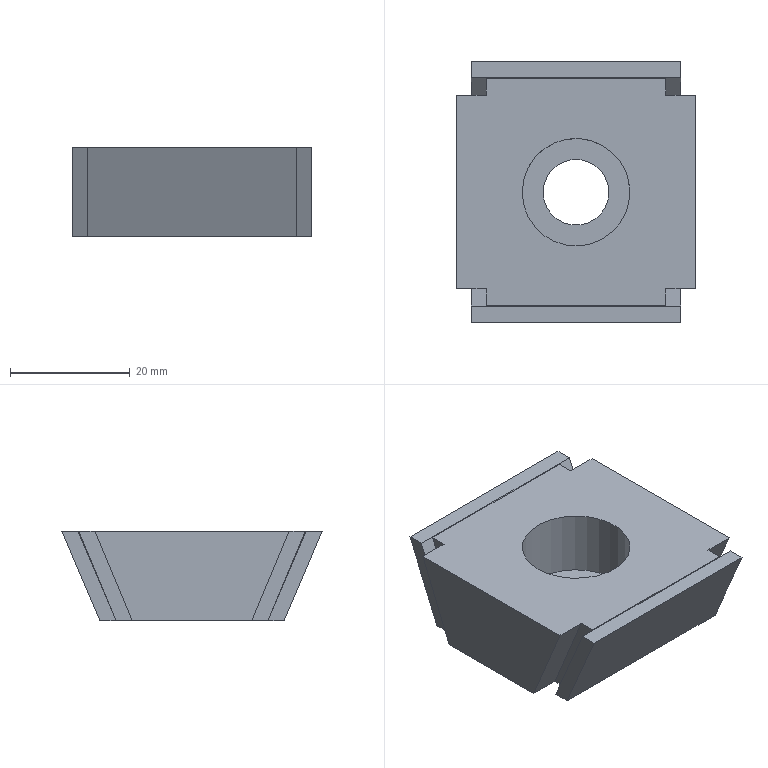Part | NX | features DATUM_CSYS 5, SKETCH 4, EXTRUDE 3, CBORE_HOLE 1, HOLE PACKAGE 1 | 3 solids | 29 faces | box 40 x 43.514 x 15 mm | volume 17811 mm3 | plane 27 | cylinder 2 | commonest cylinder face diameters 11 x1 18 x1
STEP:
#1=CARTESIAN_POINT('',(-40.,0.,0.));
#2=VERTEX_POINT('',#1);
#3=CARTESIAN_POINT('',(-35.,0.,0.));
#4=VERTEX_POINT('',#3);
#5=CARTESIAN_POINT('',(-40.,0.,0.));
#6=DIRECTION('',(1.,0.,0.));
#7=VECTOR('',#6,1000.);
#8=LINE('',#5,#7);
#9=EDGE_CURVE('',#2,#4,#8,.T.);
#10=ORIENTED_EDGE('',*,*,#9,.T.);
#11=CARTESIAN_POINT('',(-35.,-6.213,15.));
#12=VERTEX_POINT('',#11);
#13=CARTESIAN_POINT('',(-35.,0.,0.));
#14=DIRECTION('',(0.,-0.3827,0.9239));
#15=VECTOR('',#14,1000.);
#16=LINE('',#13,#15);
#17=EDGE_CURVE('',#4,#12,#16,.T.);
#18=ORIENTED_EDGE('',*,*,#17,.T.);
#19=CARTESIAN_POINT('',(-40.,-6.213,15.));
#20=VERTEX_POINT('',#19);
#21=CARTESIAN_POINT('',(-40.,-6.213,15.));
#22=DIRECTION('',(1.,0.,0.));
#23=VECTOR('',#22,1000.);
#24=LINE('',#21,#23);
#25=EDGE_CURVE('',#20,#12,#24,.T.);
#26=ORIENTED_EDGE('',*,*,#25,.F.);
#27=CARTESIAN_POINT('',(-40.,-6.213,15.));
#28=DIRECTION('',(0.,0.3827,-0.9239));
#29=VECTOR('',#28,1000.);
#30=LINE('',#27,#29);
#31=EDGE_CURVE('',#20,#2,#30,.T.);
#32=ORIENTED_EDGE('',*,*,#31,.T.);
#33=EDGE_LOOP('',(#10,#18,#26,#32));
#34=FACE_BOUND('',#33,.T.);
#35=CARTESIAN_POINT('',(-40.,-6.213,15.));
#36=DIRECTION('',(0.,-0.9239,-0.3827));
#37=DIRECTION('',(0.,0.3827,-0.9239));
#38=AXIS2_PLACEMENT_3D('',#35,#36,#37);
#39=PLANE('',#38);
#40=ADVANCED_FACE('',(#34),#39,.T.);
#41=CARTESIAN_POINT('',(-40.,26.213,15.));
#42=VERTEX_POINT('',#41);
#43=CARTESIAN_POINT('',(-35.,26.213,15.));
#44=VERTEX_POINT('',#43);
#45=CARTESIAN_POINT('',(-40.,26.213,15.));
#46=DIRECTION('',(1.,0.,0.));
#47=VECTOR('',#46,1000.);
#48=LINE('',#45,#47);
#49=EDGE_CURVE('',#42,#44,#48,.T.);
#50=ORIENTED_EDGE('',*,*,#49,.T.);
#51=CARTESIAN_POINT('',(-35.,20.,0.));
#52=VERTEX_POINT('',#51);
#53=CARTESIAN_POINT('',(-35.,26.213,15.));
#54=DIRECTION('',(0.,-0.3827,-0.9239));
#55=VECTOR('',#54,1000.);
#56=LINE('',#53,#55);
#57=EDGE_CURVE('',#44,#52,#56,.T.);
#58=ORIENTED_EDGE('',*,*,#57,.T.);
#59=CARTESIAN_POINT('',(-40.,20.,0.));
#60=VERTEX_POINT('',#59);
#61=CARTESIAN_POINT('',(-40.,20.,0.));
#62=DIRECTION('',(1.,0.,0.));
#63=VECTOR('',#62,1000.);
#64=LINE('',#61,#63);
#65=EDGE_CURVE('',#60,#52,#64,.T.);
#66=ORIENTED_EDGE('',*,*,#65,.F.);
#67=CARTESIAN_POINT('',(-40.,20.,0.));
#68=DIRECTION('',(0.,0.3827,0.9239));
#69=VECTOR('',#68,1000.);
#70=LINE('',#67,#69);
#71=EDGE_CURVE('',#60,#42,#70,.T.);
#72=ORIENTED_EDGE('',*,*,#71,.T.);
#73=EDGE_LOOP('',(#50,#58,#66,#72));
#74=FACE_BOUND('',#73,.T.);
#75=CARTESIAN_POINT('',(-40.,20.,0.));
#76=DIRECTION('',(0.,0.9239,-0.3827));
#77=DIRECTION('',(0.,0.3827,0.9239));
#78=AXIS2_PLACEMENT_3D('',#75,#76,#77);
#79=PLANE('',#78);
#80=ADVANCED_FACE('',(#74),#79,.T.);
#81=CARTESIAN_POINT('',(-5.,0.,0.));
#82=VERTEX_POINT('',#81);
#83=CARTESIAN_POINT('',(-5.,-6.213,15.));
#84=VERTEX_POINT('',#83);
#85=CARTESIAN_POINT('',(-5.,0.,0.));
#86=DIRECTION('',(0.,-0.3827,0.9239));
#87=VECTOR('',#86,1000.);
#88=LINE('',#85,#87);
#89=EDGE_CURVE('',#82,#84,#88,.T.);
#90=ORIENTED_EDGE('',*,*,#89,.F.);
#91=CARTESIAN_POINT('',(0.,0.,0.));
#92=VERTEX_POINT('',#91);
#93=CARTESIAN_POINT('',(-40.,0.,0.));
#94=DIRECTION('',(1.,0.,0.));
#95=VECTOR('',#94,1000.);
#96=LINE('',#93,#95);
#97=EDGE_CURVE('',#82,#92,#96,.T.);
#98=ORIENTED_EDGE('',*,*,#97,.T.);
#99=CARTESIAN_POINT('',(0.,-6.213,15.));
#100=VERTEX_POINT('',#99);
#101=CARTESIAN_POINT('',(0.,-6.213,15.));
#102=DIRECTION('',(0.,0.3827,-0.9239));
#103=VECTOR('',#102,1000.);
#104=LINE('',#101,#103);
#105=EDGE_CURVE('',#100,#92,#104,.T.);
#106=ORIENTED_EDGE('',*,*,#105,.F.);
#107=CARTESIAN_POINT('',(-40.,-6.213,15.));
#108=DIRECTION('',(1.,0.,0.));
#109=VECTOR('',#108,1000.);
#110=LINE('',#107,#109);
#111=EDGE_CURVE('',#84,#100,#110,.T.);
#112=ORIENTED_EDGE('',*,*,#111,.F.);
#113=EDGE_LOOP('',(#90,#98,#106,#112));
#114=FACE_BOUND('',#113,.T.);
#115=CARTESIAN_POINT('',(-40.,-6.213,15.));
#116=DIRECTION('',(0.,-0.9239,-0.3827));
#117=DIRECTION('',(0.,0.3827,-0.9239));
#118=AXIS2_PLACEMENT_3D('',#115,#116,#117);
#119=PLANE('',#118);
#120=ADVANCED_FACE('',(#114),#119,.T.);
#121=CARTESIAN_POINT('',(-25.5,9.963,0.));
#122=VERTEX_POINT('',#121);
#123=CARTESIAN_POINT('',(-20.,9.963,0.));
#124=DIRECTION('',(0.,0.,-1.));
#125=DIRECTION('',(-1.,0.,0.));
#126=AXIS2_PLACEMENT_3D('',#123,#124,#125);
#127=CIRCLE('',#126,5.5);
#128=EDGE_CURVE('',#122,#122,#127,.T.);
#129=ORIENTED_EDGE('',*,*,#128,.F.);
#130=EDGE_LOOP('',(#129));
#131=FACE_BOUND('',#130,.T.);
#132=CARTESIAN_POINT('',(0.,20.,0.));
#133=VERTEX_POINT('',#132);
#134=CARTESIAN_POINT('',(0.,0.,0.));
#135=DIRECTION('',(0.,1.,0.));
#136=VECTOR('',#135,1000.);
#137=LINE('',#134,#136);
#138=EDGE_CURVE('',#92,#133,#137,.T.);
#139=ORIENTED_EDGE('',*,*,#138,.F.);
#140=ORIENTED_EDGE('',*,*,#97,.F.);
#141=CARTESIAN_POINT('',(-5.,-2.7,0.));
#142=VERTEX_POINT('',#141);
#143=CARTESIAN_POINT('',(-5.,-2.7,0.));
#144=DIRECTION('',(0.,1.,0.));
#145=VECTOR('',#144,1000.);
#146=LINE('',#143,#145);
#147=EDGE_CURVE('',#142,#82,#146,.T.);
#148=ORIENTED_EDGE('',*,*,#147,.F.);
#149=CARTESIAN_POINT('',(-35.,-2.7,0.));
#150=VERTEX_POINT('',#149);
#151=CARTESIAN_POINT('',(-35.,-2.7,0.));
#152=DIRECTION('',(1.,0.,0.));
#153=VECTOR('',#152,1000.);
#154=LINE('',#151,#153);
#155=EDGE_CURVE('',#150,#142,#154,.T.);
#156=ORIENTED_EDGE('',*,*,#155,.F.);
#157=CARTESIAN_POINT('',(-35.,-2.7,0.));
#158=DIRECTION('',(0.,1.,0.));
#159=VECTOR('',#158,1000.);
#160=LINE('',#157,#159);
#161=EDGE_CURVE('',#150,#4,#160,.T.);
#162=ORIENTED_EDGE('',*,*,#161,.T.);
#163=ORIENTED_EDGE('',*,*,#9,.F.);
#164=CARTESIAN_POINT('',(-40.,0.,0.));
#165=DIRECTION('',(0.,1.,0.));
#166=VECTOR('',#165,1000.);
#167=LINE('',#164,#166);
#168=EDGE_CURVE('',#2,#60,#167,.T.);
#169=ORIENTED_EDGE('',*,*,#168,.T.);
#170=ORIENTED_EDGE('',*,*,#65,.T.);
#171=CARTESIAN_POINT('',(-35.,22.7,0.));
#172=VERTEX_POINT('',#171);
#173=CARTESIAN_POINT('',(-35.,20.,0.));
#174=DIRECTION('',(0.,1.,0.));
#175=VECTOR('',#174,1000.);
#176=LINE('',#173,#175);
#177=EDGE_CURVE('',#52,#172,#176,.T.);
#178=ORIENTED_EDGE('',*,*,#177,.T.);
#179=CARTESIAN_POINT('',(-5.,22.7,0.));
#180=VERTEX_POINT('',#179);
#181=CARTESIAN_POINT('',(-35.,22.7,0.));
#182=DIRECTION('',(1.,0.,0.));
#183=VECTOR('',#182,1000.);
#184=LINE('',#181,#183);
#185=EDGE_CURVE('',#172,#180,#184,.T.);
#186=ORIENTED_EDGE('',*,*,#185,.T.);
#187=CARTESIAN_POINT('',(-5.,20.,0.));
#188=VERTEX_POINT('',#187);
#189=CARTESIAN_POINT('',(-5.,20.,0.));
#190=DIRECTION('',(0.,1.,0.));
#191=VECTOR('',#190,1000.);
#192=LINE('',#189,#191);
#193=EDGE_CURVE('',#188,#180,#192,.T.);
#194=ORIENTED_EDGE('',*,*,#193,.F.);
#195=CARTESIAN_POINT('',(-40.,20.,0.));
#196=DIRECTION('',(1.,0.,0.));
#197=VECTOR('',#196,1000.);
#198=LINE('',#195,#197);
#199=EDGE_CURVE('',#188,#133,#198,.T.);
#200=ORIENTED_EDGE('',*,*,#199,.T.);
#201=EDGE_LOOP('',(#139,#140,#148,#156,#162,#163,#169,#170,#178,#186,#194,#200));
#202=FACE_BOUND('',#201,.T.);
#203=CARTESIAN_POINT('',(-40.,0.,0.));
#204=DIRECTION('',(0.,0.,-1.));
#205=DIRECTION('',(-1.,0.,0.));
#206=AXIS2_PLACEMENT_3D('',#203,#204,#205);
#207=PLANE('',#206);
#208=ADVANCED_FACE('',(#131,#202),#207,.T.);
#209=CARTESIAN_POINT('',(-5.,26.213,15.));
#210=VERTEX_POINT('',#209);
#211=CARTESIAN_POINT('',(-5.,26.213,15.));
#212=DIRECTION('',(0.,-0.3827,-0.9239));
#213=VECTOR('',#212,1000.);
#214=LINE('',#211,#213);
#215=EDGE_CURVE('',#210,#188,#214,.T.);
#216=ORIENTED_EDGE('',*,*,#215,.F.);
#217=CARTESIAN_POINT('',(0.,26.213,15.));
#218=VERTEX_POINT('',#217);
#219=CARTESIAN_POINT('',(-40.,26.213,15.));
#220=DIRECTION('',(1.,0.,0.));
#221=VECTOR('',#220,1000.);
#222=LINE('',#219,#221);
#223=EDGE_CURVE('',#210,#218,#222,.T.);
#224=ORIENTED_EDGE('',*,*,#223,.T.);
#225=CARTESIAN_POINT('',(0.,20.,0.));
#226=DIRECTION('',(0.,0.3827,0.9239));
#227=VECTOR('',#226,1000.);
#228=LINE('',#225,#227);
#229=EDGE_CURVE('',#133,#218,#228,.T.);
#230=ORIENTED_EDGE('',*,*,#229,.F.);
#231=ORIENTED_EDGE('',*,*,#199,.F.);
#232=EDGE_LOOP('',(#216,#224,#230,#231));
#233=FACE_BOUND('',#232,.T.);
#234=CARTESIAN_POINT('',(-40.,20.,0.));
#235=DIRECTION('',(0.,0.9239,-0.3827));
#236=DIRECTION('',(0.,0.3827,0.9239));
#237=AXIS2_PLACEMENT_3D('',#234,#235,#236);
#238=PLANE('',#237);
#239=ADVANCED_FACE('',(#233),#238,.T.);
#240=CARTESIAN_POINT('',(-29.,9.963,15.));
#241=VERTEX_POINT('',#240);
#242=CARTESIAN_POINT('',(-20.,9.963,15.));
#243=DIRECTION('',(0.,0.,-1.));
#244=DIRECTION('',(-1.,0.,0.));
#245=AXIS2_PLACEMENT_3D('',#242,#243,#244);
#246=CIRCLE('',#245,9.);
#247=EDGE_CURVE('',#241,#241,#246,.T.);
#248=ORIENTED_EDGE('',*,*,#247,.T.);
#249=EDGE_LOOP('',(#248));
#250=FACE_BOUND('',#249,.T.);
#251=CARTESIAN_POINT('',(0.,26.213,15.));
#252=DIRECTION('',(0.,-1.,0.));
#253=VECTOR('',#252,1000.);
#254=LINE('',#251,#253);
#255=EDGE_CURVE('',#218,#100,#254,.T.);
#256=ORIENTED_EDGE('',*,*,#255,.F.);
#257=ORIENTED_EDGE('',*,*,#223,.F.);
#258=CARTESIAN_POINT('',(-5.,28.913,15.));
#259=VERTEX_POINT('',#258);
#260=CARTESIAN_POINT('',(-5.,28.913,15.));
#261=DIRECTION('',(0.,-1.,0.));
#262=VECTOR('',#261,1000.);
#263=LINE('',#260,#262);
#264=EDGE_CURVE('',#259,#210,#263,.T.);
#265=ORIENTED_EDGE('',*,*,#264,.F.);
#266=CARTESIAN_POINT('',(-35.,28.913,15.));
#267=VERTEX_POINT('',#266);
#268=CARTESIAN_POINT('',(-35.,28.913,15.));
#269=DIRECTION('',(1.,0.,0.));
#270=VECTOR('',#269,1000.);
#271=LINE('',#268,#270);
#272=EDGE_CURVE('',#267,#259,#271,.T.);
#273=ORIENTED_EDGE('',*,*,#272,.F.);
#274=CARTESIAN_POINT('',(-35.,28.913,15.));
#275=DIRECTION('',(0.,-1.,0.));
#276=VECTOR('',#275,1000.);
#277=LINE('',#274,#276);
#278=EDGE_CURVE('',#267,#44,#277,.T.);
#279=ORIENTED_EDGE('',*,*,#278,.T.);
#280=ORIENTED_EDGE('',*,*,#49,.F.);
#281=CARTESIAN_POINT('',(-40.,26.213,15.));
#282=DIRECTION('',(0.,-1.,0.));
#283=VECTOR('',#282,1000.);
#284=LINE('',#281,#283);
#285=EDGE_CURVE('',#42,#20,#284,.T.);
#286=ORIENTED_EDGE('',*,*,#285,.T.);
#287=ORIENTED_EDGE('',*,*,#25,.T.);
#288=CARTESIAN_POINT('',(-35.,-8.913,15.));
#289=VERTEX_POINT('',#288);
#290=CARTESIAN_POINT('',(-35.,-6.213,15.));
#291=DIRECTION('',(0.,-1.,0.));
#292=VECTOR('',#291,1000.);
#293=LINE('',#290,#292);
#294=EDGE_CURVE('',#12,#289,#293,.T.);
#295=ORIENTED_EDGE('',*,*,#294,.T.);
#296=CARTESIAN_POINT('',(-5.,-8.913,15.));
#297=VERTEX_POINT('',#296);
#298=CARTESIAN_POINT('',(-35.,-8.913,15.));
#299=DIRECTION('',(1.,0.,0.));
#300=VECTOR('',#299,1000.);
#301=LINE('',#298,#300);
#302=EDGE_CURVE('',#289,#297,#301,.T.);
#303=ORIENTED_EDGE('',*,*,#302,.T.);
#304=CARTESIAN_POINT('',(-5.,-6.213,15.));
#305=DIRECTION('',(0.,-1.,0.));
#306=VECTOR('',#305,1000.);
#307=LINE('',#304,#306);
#308=EDGE_CURVE('',#84,#297,#307,.T.);
#309=ORIENTED_EDGE('',*,*,#308,.F.);
#310=ORIENTED_EDGE('',*,*,#111,.T.);
#311=EDGE_LOOP('',(#256,#257,#265,#273,#279,#280,#286,#287,#295,#303,#309,#310));
#312=FACE_BOUND('',#311,.T.);
#313=CARTESIAN_POINT('',(-40.,26.213,15.));
#314=DIRECTION('',(0.,0.,1.));
#315=DIRECTION('',(1.,0.,0.));
#316=AXIS2_PLACEMENT_3D('',#313,#314,#315);
#317=PLANE('',#316);
#318=ADVANCED_FACE('',(#250,#312),#317,.T.);
#319=ORIENTED_EDGE('',*,*,#31,.F.);
#320=ORIENTED_EDGE('',*,*,#285,.F.);
#321=ORIENTED_EDGE('',*,*,#71,.F.);
#322=ORIENTED_EDGE('',*,*,#168,.F.);
#323=EDGE_LOOP('',(#319,#320,#321,#322));
#324=FACE_BOUND('',#323,.T.);
#325=CARTESIAN_POINT('',(-40.,0.,0.));
#326=DIRECTION('',(1.,0.,0.));
#327=DIRECTION('',(0.,0.,-1.));
#328=AXIS2_PLACEMENT_3D('',#325,#326,#327);
#329=PLANE('',#328);
#330=ADVANCED_FACE('',(#324),#329,.F.);
#331=ORIENTED_EDGE('',*,*,#105,.T.);
#332=ORIENTED_EDGE('',*,*,#138,.T.);
#333=ORIENTED_EDGE('',*,*,#229,.T.);
#334=ORIENTED_EDGE('',*,*,#255,.T.);
#335=EDGE_LOOP('',(#331,#332,#333,#334));
#336=FACE_BOUND('',#335,.T.);
#337=CARTESIAN_POINT('',(0.,0.,0.));
#338=DIRECTION('',(1.,0.,0.));
#339=DIRECTION('',(0.,0.,-1.));
#340=AXIS2_PLACEMENT_3D('',#337,#338,#339);
#341=PLANE('',#340);
#342=ADVANCED_FACE('',(#336),#341,.T.);
#343=CARTESIAN_POINT('',(-5.,22.7,0.));
#344=DIRECTION('',(0.,0.3827,0.9239));
#345=VECTOR('',#344,1000.);
#346=LINE('',#343,#345);
#347=EDGE_CURVE('',#180,#259,#346,.T.);
#348=ORIENTED_EDGE('',*,*,#347,.F.);
#349=ORIENTED_EDGE('',*,*,#185,.F.);
#350=CARTESIAN_POINT('',(-35.,22.7,0.));
#351=DIRECTION('',(0.,0.3827,0.9239));
#352=VECTOR('',#351,1000.);
#353=LINE('',#350,#352);
#354=EDGE_CURVE('',#172,#267,#353,.T.);
#355=ORIENTED_EDGE('',*,*,#354,.T.);
#356=ORIENTED_EDGE('',*,*,#272,.T.);
#357=EDGE_LOOP('',(#348,#349,#355,#356));
#358=FACE_BOUND('',#357,.T.);
#359=CARTESIAN_POINT('',(-35.,22.7,0.));
#360=DIRECTION('',(0.,0.9239,-0.3827));
#361=DIRECTION('',(0.,0.3827,0.9239));
#362=AXIS2_PLACEMENT_3D('',#359,#360,#361);
#363=PLANE('',#362);
#364=ADVANCED_FACE('',(#358),#363,.T.);
#365=ORIENTED_EDGE('',*,*,#177,.F.);
#366=ORIENTED_EDGE('',*,*,#57,.F.);
#367=ORIENTED_EDGE('',*,*,#278,.F.);
#368=ORIENTED_EDGE('',*,*,#354,.F.);
#369=EDGE_LOOP('',(#365,#366,#367,#368));
#370=FACE_BOUND('',#369,.T.);
#371=CARTESIAN_POINT('',(-35.,0.,0.));
#372=DIRECTION('',(1.,0.,0.));
#373=DIRECTION('',(0.,0.,-1.));
#374=AXIS2_PLACEMENT_3D('',#371,#372,#373);
#375=PLANE('',#374);
#376=ADVANCED_FACE('',(#370),#375,.F.);
#377=ORIENTED_EDGE('',*,*,#193,.T.);
#378=ORIENTED_EDGE('',*,*,#347,.T.);
#379=ORIENTED_EDGE('',*,*,#264,.T.);
#380=ORIENTED_EDGE('',*,*,#215,.T.);
#381=EDGE_LOOP('',(#377,#378,#379,#380));
#382=FACE_BOUND('',#381,.T.);
#383=CARTESIAN_POINT('',(-5.,0.,0.));
#384=DIRECTION('',(1.,0.,0.));
#385=DIRECTION('',(0.,0.,-1.));
#386=AXIS2_PLACEMENT_3D('',#383,#384,#385);
#387=PLANE('',#386);
#388=ADVANCED_FACE('',(#382),#387,.T.);
#389=CARTESIAN_POINT('',(-5.,-8.913,15.));
#390=DIRECTION('',(0.,0.3827,-0.9239));
#391=VECTOR('',#390,1000.);
#392=LINE('',#389,#391);
#393=EDGE_CURVE('',#297,#142,#392,.T.);
#394=ORIENTED_EDGE('',*,*,#393,.F.);
#395=ORIENTED_EDGE('',*,*,#302,.F.);
#396=CARTESIAN_POINT('',(-35.,-8.913,15.));
#397=DIRECTION('',(0.,0.3827,-0.9239));
#398=VECTOR('',#397,1000.);
#399=LINE('',#396,#398);
#400=EDGE_CURVE('',#289,#150,#399,.T.);
#401=ORIENTED_EDGE('',*,*,#400,.T.);
#402=ORIENTED_EDGE('',*,*,#155,.T.);
#403=EDGE_LOOP('',(#394,#395,#401,#402));
#404=FACE_BOUND('',#403,.T.);
#405=CARTESIAN_POINT('',(-35.,-8.913,15.));
#406=DIRECTION('',(0.,-0.9239,-0.3827));
#407=DIRECTION('',(0.,0.3827,-0.9239));
#408=AXIS2_PLACEMENT_3D('',#405,#406,#407);
#409=PLANE('',#408);
#410=ADVANCED_FACE('',(#404),#409,.T.);
#411=ORIENTED_EDGE('',*,*,#294,.F.);
#412=ORIENTED_EDGE('',*,*,#17,.F.);
#413=ORIENTED_EDGE('',*,*,#161,.F.);
#414=ORIENTED_EDGE('',*,*,#400,.F.);
#415=EDGE_LOOP('',(#411,#412,#413,#414));
#416=FACE_BOUND('',#415,.T.);
#417=CARTESIAN_POINT('',(-35.,0.,0.));
#418=DIRECTION('',(1.,0.,0.));
#419=DIRECTION('',(0.,0.,-1.));
#420=AXIS2_PLACEMENT_3D('',#417,#418,#419);
#421=PLANE('',#420);
#422=ADVANCED_FACE('',(#416),#421,.F.);
#423=ORIENTED_EDGE('',*,*,#308,.T.);
#424=ORIENTED_EDGE('',*,*,#393,.T.);
#425=ORIENTED_EDGE('',*,*,#147,.T.);
#426=ORIENTED_EDGE('',*,*,#89,.T.);
#427=EDGE_LOOP('',(#423,#424,#425,#426));
#428=FACE_BOUND('',#427,.T.);
#429=CARTESIAN_POINT('',(-5.,0.,0.));
#430=DIRECTION('',(1.,0.,0.));
#431=DIRECTION('',(0.,0.,-1.));
#432=AXIS2_PLACEMENT_3D('',#429,#430,#431);
#433=PLANE('',#432);
#434=ADVANCED_FACE('',(#428),#433,.T.);
#435=ORIENTED_EDGE('',*,*,#128,.T.);
#436=EDGE_LOOP('',(#435));
#437=FACE_BOUND('',#436,.T.);
#438=CARTESIAN_POINT('',(-25.5,9.963,4.));
#439=VERTEX_POINT('',#438);
#440=CARTESIAN_POINT('',(-20.,9.963,4.));
#441=DIRECTION('',(0.,0.,-1.));
#442=DIRECTION('',(-1.,0.,0.));
#443=AXIS2_PLACEMENT_3D('',#440,#441,#442);
#444=CIRCLE('',#443,5.5);
#445=EDGE_CURVE('',#439,#439,#444,.F.);
#446=ORIENTED_EDGE('',*,*,#445,.T.);
#447=EDGE_LOOP('',(#446));
#448=FACE_BOUND('',#447,.T.);
#449=CARTESIAN_POINT('',(-20.,9.963,-35.));
#450=DIRECTION('',(0.,0.,-1.));
#451=DIRECTION('',(-1.,0.,0.));
#452=AXIS2_PLACEMENT_3D('',#449,#450,#451);
#453=CYLINDRICAL_SURFACE('',#452,5.5);
#454=ADVANCED_FACE('',(#437,#448),#453,.F.);
#455=ORIENTED_EDGE('',*,*,#445,.F.);
#456=EDGE_LOOP('',(#455));
#457=FACE_BOUND('',#456,.T.);
#458=CARTESIAN_POINT('',(-29.,9.963,4.));
#459=VERTEX_POINT('',#458);
#460=CARTESIAN_POINT('',(-20.,9.963,4.));
#461=DIRECTION('',(0.,0.,-1.));
#462=DIRECTION('',(-1.,0.,0.));
#463=AXIS2_PLACEMENT_3D('',#460,#461,#462);
#464=CIRCLE('',#463,9.);
#465=EDGE_CURVE('',#459,#459,#464,.F.);
#466=ORIENTED_EDGE('',*,*,#465,.T.);
#467=EDGE_LOOP('',(#466));
#468=FACE_BOUND('',#467,.T.);
#469=CARTESIAN_POINT('',(-20.,9.963,4.));
#470=DIRECTION('',(0.,0.,-1.));
#471=DIRECTION('',(-1.,0.,0.));
#472=AXIS2_PLACEMENT_3D('',#469,#470,#471);
#473=PLANE('',#472);
#474=ADVANCED_FACE('',(#457,#468),#473,.F.);
#475=ORIENTED_EDGE('',*,*,#465,.F.);
#476=EDGE_LOOP('',(#475));
#477=FACE_BOUND('',#476,.T.);
#478=ORIENTED_EDGE('',*,*,#247,.F.);
#479=EDGE_LOOP('',(#478));
#480=FACE_BOUND('',#479,.T.);
#481=CARTESIAN_POINT('',(-20.,9.963,15.));
#482=DIRECTION('',(0.,0.,-1.));
#483=DIRECTION('',(-1.,0.,0.));
#484=AXIS2_PLACEMENT_3D('',#481,#482,#483);
#485=CYLINDRICAL_SURFACE('',#484,9.);
#486=ADVANCED_FACE('',(#477,#480),#485,.F.);
#487=CLOSED_SHELL('',(#40,#80,#120,#208,#239,#318,#330,#342,#364,#376,#388,#410,#422,#434,#454,#474,#486));
#488=MANIFOLD_SOLID_BREP('',#487);
#489=CARTESIAN_POINT('',(-2.5,-9.067,15.));
#490=VERTEX_POINT('',#489);
#491=CARTESIAN_POINT('',(-2.5,-11.757,14.977));
#492=VERTEX_POINT('',#491);
#493=CARTESIAN_POINT('',(-2.5,-9.067,15.));
#494=DIRECTION('',(0.,-1.,-0.008727));
#495=VECTOR('',#494,1000.);
#496=LINE('',#493,#495);
#497=EDGE_CURVE('',#490,#492,#496,.T.);
#498=ORIENTED_EDGE('',*,*,#497,.F.);
#499=CARTESIAN_POINT('',(-37.5,-9.067,15.));
#500=VERTEX_POINT('',#499);
#501=CARTESIAN_POINT('',(-37.5,-9.067,15.));
#502=DIRECTION('',(1.,0.,0.));
#503=VECTOR('',#502,1000.);
#504=LINE('',#501,#503);
#505=EDGE_CURVE('',#500,#490,#504,.T.);
#506=ORIENTED_EDGE('',*,*,#505,.F.);
#507=CARTESIAN_POINT('',(-37.5,-11.757,14.977));
#508=VERTEX_POINT('',#507);
#509=CARTESIAN_POINT('',(-37.5,-9.067,15.));
#510=DIRECTION('',(0.,-1.,-0.008727));
#511=VECTOR('',#510,1000.);
#512=LINE('',#509,#511);
#513=EDGE_CURVE('',#500,#508,#512,.T.);
#514=ORIENTED_EDGE('',*,*,#513,.T.);
#515=CARTESIAN_POINT('',(-37.5,-11.757,14.977));
#516=DIRECTION('',(1.,0.,0.));
#517=VECTOR('',#516,1000.);
#518=LINE('',#515,#517);
#519=EDGE_CURVE('',#508,#492,#518,.T.);
#520=ORIENTED_EDGE('',*,*,#519,.T.);
#521=EDGE_LOOP('',(#498,#506,#514,#520));
#522=FACE_BOUND('',#521,.T.);
#523=CARTESIAN_POINT('',(-37.5,-9.067,15.));
#524=DIRECTION('',(0.,-0.008727,1.));
#525=DIRECTION('',(0.,-1.,-0.008727));
#526=AXIS2_PLACEMENT_3D('',#523,#524,#525);
#527=PLANE('',#526);
#528=ADVANCED_FACE('',(#522),#527,.T.);
#529=CARTESIAN_POINT('',(-2.5,-5.4,0.));
#530=VERTEX_POINT('',#529);
#531=CARTESIAN_POINT('',(-2.5,-11.757,14.977));
#532=DIRECTION('',(0.,0.3907,-0.9205));
#533=VECTOR('',#532,1000.);
#534=LINE('',#531,#533);
#535=EDGE_CURVE('',#492,#530,#534,.T.);
#536=ORIENTED_EDGE('',*,*,#535,.F.);
#537=ORIENTED_EDGE('',*,*,#519,.F.);
#538=CARTESIAN_POINT('',(-37.5,-5.4,0.));
#539=VERTEX_POINT('',#538);
#540=CARTESIAN_POINT('',(-37.5,-11.757,14.977));
#541=DIRECTION('',(0.,0.3907,-0.9205));
#542=VECTOR('',#541,1000.);
#543=LINE('',#540,#542);
#544=EDGE_CURVE('',#508,#539,#543,.T.);
#545=ORIENTED_EDGE('',*,*,#544,.T.);
#546=CARTESIAN_POINT('',(-37.5,-5.4,0.));
#547=DIRECTION('',(1.,0.,0.));
#548=VECTOR('',#547,1000.);
#549=LINE('',#546,#548);
#550=EDGE_CURVE('',#539,#530,#549,.T.);
#551=ORIENTED_EDGE('',*,*,#550,.T.);
#552=EDGE_LOOP('',(#536,#537,#545,#551));
#553=FACE_BOUND('',#552,.T.);
#554=CARTESIAN_POINT('',(-37.5,-11.757,14.977));
#555=DIRECTION('',(0.,-0.9205,-0.3907));
#556=DIRECTION('',(0.,0.3907,-0.9205));
#557=AXIS2_PLACEMENT_3D('',#554,#555,#556);
#558=PLANE('',#557);
#559=ADVANCED_FACE('',(#553),#558,.T.);
#560=CARTESIAN_POINT('',(-2.5,-2.7,0.));
#561=VERTEX_POINT('',#560);
#562=CARTESIAN_POINT('',(-2.5,-5.4,0.));
#563=DIRECTION('',(0.,1.,0.));
#564=VECTOR('',#563,1000.);
#565=LINE('',#562,#564);
#566=EDGE_CURVE('',#530,#561,#565,.T.);
#567=ORIENTED_EDGE('',*,*,#566,.F.);
#568=ORIENTED_EDGE('',*,*,#550,.F.);
#569=CARTESIAN_POINT('',(-37.5,-2.7,0.));
#570=VERTEX_POINT('',#569);
#571=CARTESIAN_POINT('',(-37.5,-5.4,0.));
#572=DIRECTION('',(0.,1.,0.));
#573=VECTOR('',#572,1000.);
#574=LINE('',#571,#573);
#575=EDGE_CURVE('',#539,#570,#574,.T.);
#576=ORIENTED_EDGE('',*,*,#575,.T.);
#577=CARTESIAN_POINT('',(-37.5,-2.7,0.));
#578=DIRECTION('',(1.,0.,0.));
#579=VECTOR('',#578,1000.);
#580=LINE('',#577,#579);
#581=EDGE_CURVE('',#570,#561,#580,.T.);
#582=ORIENTED_EDGE('',*,*,#581,.T.);
#583=EDGE_LOOP('',(#567,#568,#576,#582));
#584=FACE_BOUND('',#583,.T.);
#585=CARTESIAN_POINT('',(-37.5,-5.4,0.));
#586=DIRECTION('',(0.,0.,-1.));
#587=DIRECTION('',(0.,1.,0.));
#588=AXIS2_PLACEMENT_3D('',#585,#586,#587);
#589=PLANE('',#588);
#590=ADVANCED_FACE('',(#584),#589,.T.);
#591=CARTESIAN_POINT('',(-2.5,-2.7,0.));
#592=DIRECTION('',(0.,-0.3907,0.9205));
#593=VECTOR('',#592,1000.);
#594=LINE('',#591,#593);
#595=EDGE_CURVE('',#561,#490,#594,.T.);
#596=ORIENTED_EDGE('',*,*,#595,.F.);
#597=ORIENTED_EDGE('',*,*,#581,.F.);
#598=CARTESIAN_POINT('',(-37.5,-2.7,0.));
#599=DIRECTION('',(0.,-0.3907,0.9205));
#600=VECTOR('',#599,1000.);
#601=LINE('',#598,#600);
#602=EDGE_CURVE('',#570,#500,#601,.T.);
#603=ORIENTED_EDGE('',*,*,#602,.T.);
#604=ORIENTED_EDGE('',*,*,#505,.T.);
#605=EDGE_LOOP('',(#596,#597,#603,#604));
#606=FACE_BOUND('',#605,.T.);
#607=CARTESIAN_POINT('',(-37.5,-2.7,0.));
#608=DIRECTION('',(0.,0.9205,0.3907));
#609=DIRECTION('',(0.,-0.3907,0.9205));
#610=AXIS2_PLACEMENT_3D('',#607,#608,#609);
#611=PLANE('',#610);
#612=ADVANCED_FACE('',(#606),#611,.T.);
#613=ORIENTED_EDGE('',*,*,#513,.F.);
#614=ORIENTED_EDGE('',*,*,#602,.F.);
#615=ORIENTED_EDGE('',*,*,#575,.F.);
#616=ORIENTED_EDGE('',*,*,#544,.F.);
#617=EDGE_LOOP('',(#613,#614,#615,#616));
#618=FACE_BOUND('',#617,.T.);
#619=CARTESIAN_POINT('',(-37.5,0.,0.));
#620=DIRECTION('',(1.,0.,0.));
#621=DIRECTION('',(0.,0.,-1.));
#622=AXIS2_PLACEMENT_3D('',#619,#620,#621);
#623=PLANE('',#622);
#624=ADVANCED_FACE('',(#618),#623,.F.);
#625=ORIENTED_EDGE('',*,*,#497,.T.);
#626=ORIENTED_EDGE('',*,*,#535,.T.);
#627=ORIENTED_EDGE('',*,*,#566,.T.);
#628=ORIENTED_EDGE('',*,*,#595,.T.);
#629=EDGE_LOOP('',(#625,#626,#627,#628));
#630=FACE_BOUND('',#629,.T.);
#631=CARTESIAN_POINT('',(-2.5,0.,0.));
#632=DIRECTION('',(1.,0.,0.));
#633=DIRECTION('',(0.,0.,-1.));
#634=AXIS2_PLACEMENT_3D('',#631,#632,#633);
#635=PLANE('',#634);
#636=ADVANCED_FACE('',(#630),#635,.T.);
#637=CLOSED_SHELL('',(#528,#559,#590,#612,#624,#636));
#638=MANIFOLD_SOLID_BREP('',#637);
#639=CARTESIAN_POINT('',(-2.5,22.7,0.));
#640=VERTEX_POINT('',#639);
#641=CARTESIAN_POINT('',(-2.5,25.4,0.));
#642=VERTEX_POINT('',#641);
#643=CARTESIAN_POINT('',(-2.5,22.7,0.));
#644=DIRECTION('',(0.,1.,0.));
#645=VECTOR('',#644,1000.);
#646=LINE('',#643,#645);
#647=EDGE_CURVE('',#640,#642,#646,.T.);
#648=ORIENTED_EDGE('',*,*,#647,.F.);
#649=CARTESIAN_POINT('',(-37.5,22.7,0.));
#650=VERTEX_POINT('',#649);
#651=CARTESIAN_POINT('',(-37.5,22.7,0.));
#652=DIRECTION('',(1.,0.,0.));
#653=VECTOR('',#652,1000.);
#654=LINE('',#651,#653);
#655=EDGE_CURVE('',#650,#640,#654,.T.);
#656=ORIENTED_EDGE('',*,*,#655,.F.);
#657=CARTESIAN_POINT('',(-37.5,25.4,0.));
#658=VERTEX_POINT('',#657);
#659=CARTESIAN_POINT('',(-37.5,22.7,0.));
#660=DIRECTION('',(0.,1.,0.));
#661=VECTOR('',#660,1000.);
#662=LINE('',#659,#661);
#663=EDGE_CURVE('',#650,#658,#662,.T.);
#664=ORIENTED_EDGE('',*,*,#663,.T.);
#665=CARTESIAN_POINT('',(-37.5,25.4,0.));
#666=DIRECTION('',(1.,0.,0.));
#667=VECTOR('',#666,1000.);
#668=LINE('',#665,#667);
#669=EDGE_CURVE('',#658,#642,#668,.T.);
#670=ORIENTED_EDGE('',*,*,#669,.T.);
#671=EDGE_LOOP('',(#648,#656,#664,#670));
#672=FACE_BOUND('',#671,.T.);
#673=CARTESIAN_POINT('',(-37.5,22.7,0.));
#674=DIRECTION('',(0.,0.,-1.));
#675=DIRECTION('',(0.,1.,0.));
#676=AXIS2_PLACEMENT_3D('',#673,#674,#675);
#677=PLANE('',#676);
#678=ADVANCED_FACE('',(#672),#677,.T.);
#679=CARTESIAN_POINT('',(-2.5,31.757,14.977));
#680=VERTEX_POINT('',#679);
#681=CARTESIAN_POINT('',(-2.5,25.4,0.));
#682=DIRECTION('',(0.,0.3907,0.9205));
#683=VECTOR('',#682,1000.);
#684=LINE('',#681,#683);
#685=EDGE_CURVE('',#642,#680,#684,.T.);
#686=ORIENTED_EDGE('',*,*,#685,.F.);
#687=ORIENTED_EDGE('',*,*,#669,.F.);
#688=CARTESIAN_POINT('',(-37.5,31.757,14.977));
#689=VERTEX_POINT('',#688);
#690=CARTESIAN_POINT('',(-37.5,25.4,0.));
#691=DIRECTION('',(0.,0.3907,0.9205));
#692=VECTOR('',#691,1000.);
#693=LINE('',#690,#692);
#694=EDGE_CURVE('',#658,#689,#693,.T.);
#695=ORIENTED_EDGE('',*,*,#694,.T.);
#696=CARTESIAN_POINT('',(-37.5,31.757,14.977));
#697=DIRECTION('',(1.,0.,0.));
#698=VECTOR('',#697,1000.);
#699=LINE('',#696,#698);
#700=EDGE_CURVE('',#689,#680,#699,.T.);
#701=ORIENTED_EDGE('',*,*,#700,.T.);
#702=EDGE_LOOP('',(#686,#687,#695,#701));
#703=FACE_BOUND('',#702,.T.);
#704=CARTESIAN_POINT('',(-37.5,25.4,0.));
#705=DIRECTION('',(0.,0.9205,-0.3907));
#706=DIRECTION('',(0.,0.3907,0.9205));
#707=AXIS2_PLACEMENT_3D('',#704,#705,#706);
#708=PLANE('',#707);
#709=ADVANCED_FACE('',(#703),#708,.T.);
#710=CARTESIAN_POINT('',(-2.5,29.067,15.));
#711=VERTEX_POINT('',#710);
#712=CARTESIAN_POINT('',(-2.5,31.757,14.977));
#713=DIRECTION('',(0.,-1.,0.008727));
#714=VECTOR('',#713,1000.);
#715=LINE('',#712,#714);
#716=EDGE_CURVE('',#680,#711,#715,.T.);
#717=ORIENTED_EDGE('',*,*,#716,.F.);
#718=ORIENTED_EDGE('',*,*,#700,.F.);
#719=CARTESIAN_POINT('',(-37.5,29.067,15.));
#720=VERTEX_POINT('',#719);
#721=CARTESIAN_POINT('',(-37.5,31.757,14.977));
#722=DIRECTION('',(0.,-1.,0.008727));
#723=VECTOR('',#722,1000.);
#724=LINE('',#721,#723);
#725=EDGE_CURVE('',#689,#720,#724,.T.);
#726=ORIENTED_EDGE('',*,*,#725,.T.);
#727=CARTESIAN_POINT('',(-37.5,29.067,15.));
#728=DIRECTION('',(1.,0.,0.));
#729=VECTOR('',#728,1000.);
#730=LINE('',#727,#729);
#731=EDGE_CURVE('',#720,#711,#730,.T.);
#732=ORIENTED_EDGE('',*,*,#731,.T.);
#733=EDGE_LOOP('',(#717,#718,#726,#732));
#734=FACE_BOUND('',#733,.T.);
#735=CARTESIAN_POINT('',(-37.5,31.757,14.977));
#736=DIRECTION('',(0.,0.008727,1.));
#737=DIRECTION('',(0.,-1.,0.008727));
#738=AXIS2_PLACEMENT_3D('',#735,#736,#737);
#739=PLANE('',#738);
#740=ADVANCED_FACE('',(#734),#739,.T.);
#741=CARTESIAN_POINT('',(-2.5,29.067,15.));
#742=DIRECTION('',(0.,-0.3907,-0.9205));
#743=VECTOR('',#742,1000.);
#744=LINE('',#741,#743);
#745=EDGE_CURVE('',#711,#640,#744,.T.);
#746=ORIENTED_EDGE('',*,*,#745,.F.);
#747=ORIENTED_EDGE('',*,*,#731,.F.);
#748=CARTESIAN_POINT('',(-37.5,29.067,15.));
#749=DIRECTION('',(0.,-0.3907,-0.9205));
#750=VECTOR('',#749,1000.);
#751=LINE('',#748,#750);
#752=EDGE_CURVE('',#720,#650,#751,.T.);
#753=ORIENTED_EDGE('',*,*,#752,.T.);
#754=ORIENTED_EDGE('',*,*,#655,.T.);
#755=EDGE_LOOP('',(#746,#747,#753,#754));
#756=FACE_BOUND('',#755,.T.);
#757=CARTESIAN_POINT('',(-37.5,29.067,15.));
#758=DIRECTION('',(0.,-0.9205,0.3907));
#759=DIRECTION('',(0.,-0.3907,-0.9205));
#760=AXIS2_PLACEMENT_3D('',#757,#758,#759);
#761=PLANE('',#760);
#762=ADVANCED_FACE('',(#756),#761,.T.);
#763=ORIENTED_EDGE('',*,*,#663,.F.);
#764=ORIENTED_EDGE('',*,*,#752,.F.);
#765=ORIENTED_EDGE('',*,*,#725,.F.);
#766=ORIENTED_EDGE('',*,*,#694,.F.);
#767=EDGE_LOOP('',(#763,#764,#765,#766));
#768=FACE_BOUND('',#767,.T.);
#769=CARTESIAN_POINT('',(-37.5,0.,0.));
#770=DIRECTION('',(1.,0.,0.));
#771=DIRECTION('',(0.,0.,-1.));
#772=AXIS2_PLACEMENT_3D('',#769,#770,#771);
#773=PLANE('',#772);
#774=ADVANCED_FACE('',(#768),#773,.F.);
#775=ORIENTED_EDGE('',*,*,#647,.T.);
#776=ORIENTED_EDGE('',*,*,#685,.T.);
#777=ORIENTED_EDGE('',*,*,#716,.T.);
#778=ORIENTED_EDGE('',*,*,#745,.T.);
#779=EDGE_LOOP('',(#775,#776,#777,#778));
#780=FACE_BOUND('',#779,.T.);
#781=CARTESIAN_POINT('',(-2.5,0.,0.));
#782=DIRECTION('',(1.,0.,0.));
#783=DIRECTION('',(0.,0.,-1.));
#784=AXIS2_PLACEMENT_3D('',#781,#782,#783);
#785=PLANE('',#784);
#786=ADVANCED_FACE('',(#780),#785,.T.);
#787=CLOSED_SHELL('',(#678,#709,#740,#762,#774,#786));
#788=MANIFOLD_SOLID_BREP('',#787);
#789=(LENGTH_UNIT()NAMED_UNIT(*)SI_UNIT(.MILLI.,.METRE.));
#790=UNCERTAINTY_MEASURE_WITH_UNIT(LENGTH_MEASURE(0.00001),#789,'','');
#791=(NAMED_UNIT(*)PLANE_ANGLE_UNIT()SI_UNIT($,.RADIAN.));
#792=(NAMED_UNIT(*)SI_UNIT($,.STERADIAN.)SOLID_ANGLE_UNIT());
#793=(GEOMETRIC_REPRESENTATION_CONTEXT(3)GLOBAL_UNCERTAINTY_ASSIGNED_CONTEXT((#790))GLOBAL_UNIT_ASSIGNED_CONTEXT((#789,#791,#792))REPRESENTATION_CONTEXT('',''));
#794=ADVANCED_BREP_SHAPE_REPRESENTATION('',(#488,#638,#788),#793);